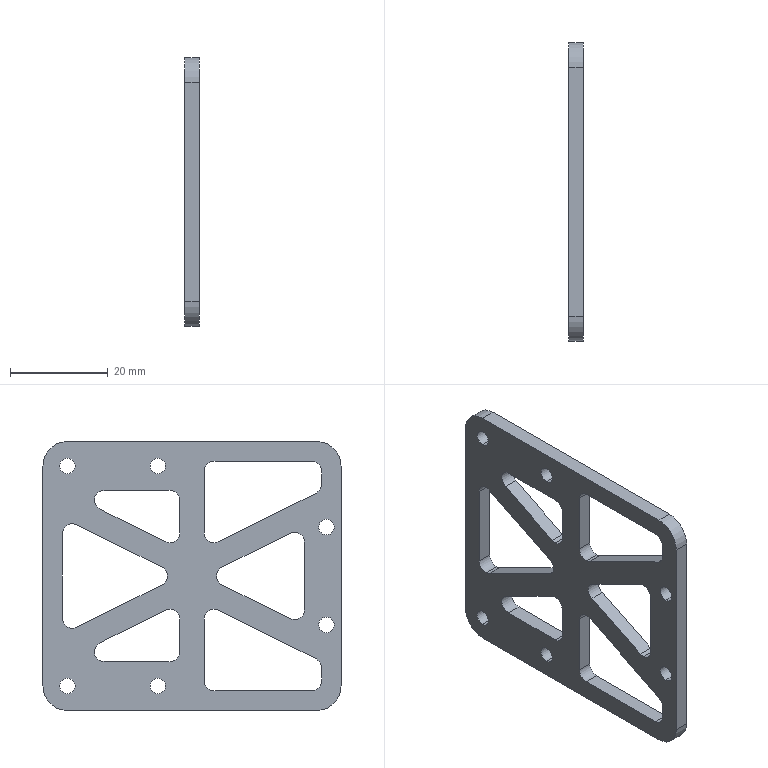Part | SolidWorks | features Fillet 2, ICE 2, Extrusion 1 | 1 solid | 66 faces | box 3 x 61 x 55 mm | volume 5958 mm3 | cylinder 40 | plane 26 | commonest cylinder face diameters 4 x24 3.2 x12 10 x4